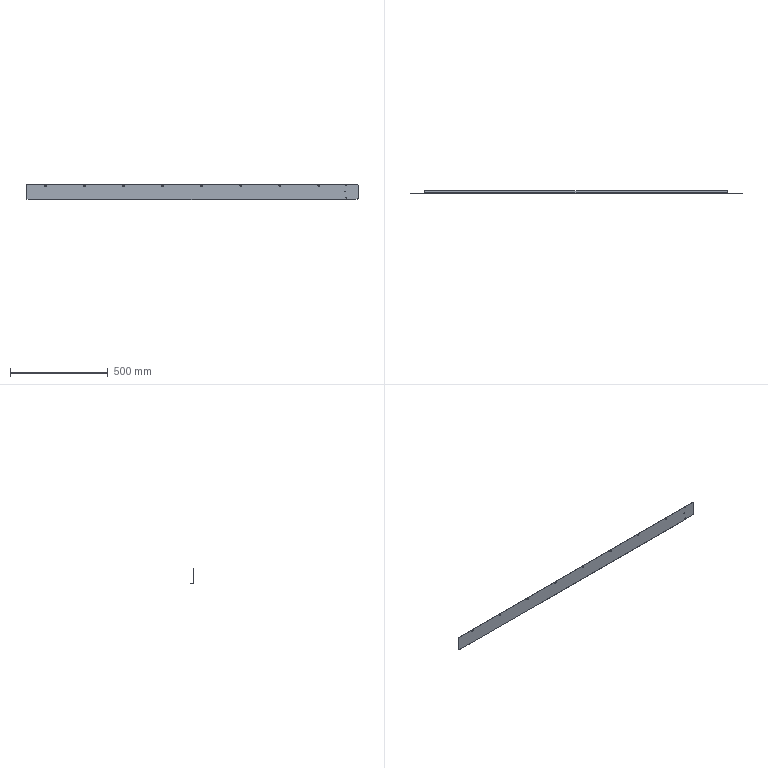Part | STEP file | 1 solid | 64 faces | box 1700 x 15 x 80 mm | volume 308828 mm3 | plane 36 | cylinder 28 | commonest cylinder face diameters 5.5 x16 3.3 x6 10 x4 1 x1 5 x1